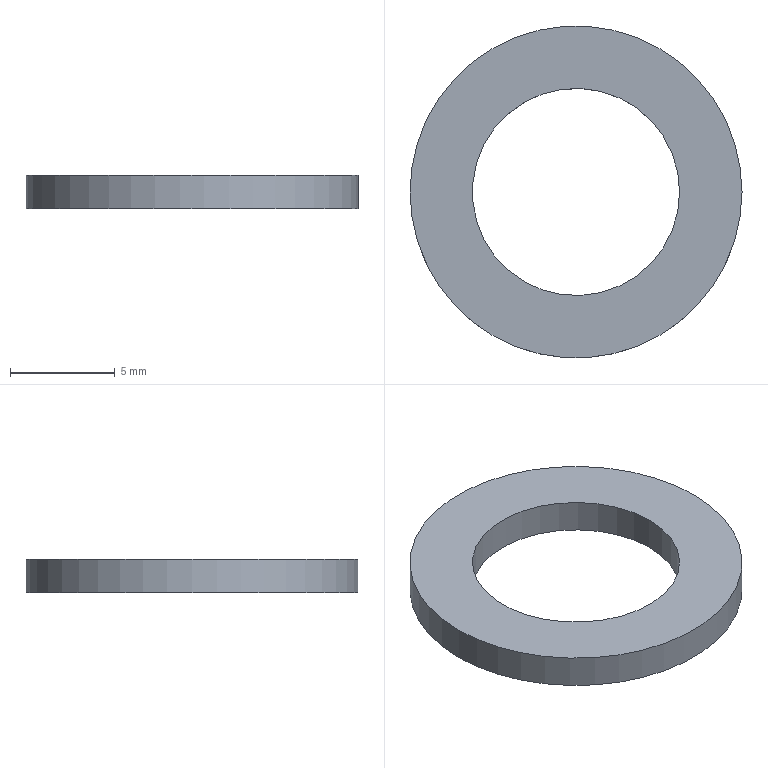Part | NX | features solid 2 | 1 solid | 4 faces | box 15.875 x 15.875 x 1.6 mm | volume 193.404 mm3 | cylinder 2 | plane 2 | commonest cylinder face diameters 9.906 x1 15.875 x1
STEP:
#1=CARTESIAN_POINT('',(7.938,0.,1.6));
#2=VERTEX_POINT('',#1);
#3=CARTESIAN_POINT('',(0.,0.,1.6));
#4=DIRECTION('',(0.,0.,-1.));
#5=DIRECTION('',(1.,0.,0.));
#6=AXIS2_PLACEMENT_3D('',#3,#4,#5);
#7=CIRCLE('',#6,7.938);
#8=EDGE_CURVE('',#2,#2,#7,.T.);
#9=ORIENTED_EDGE('',*,*,#8,.T.);
#10=EDGE_LOOP('',(#9));
#11=FACE_BOUND('',#10,.T.);
#12=CARTESIAN_POINT('',(7.938,0.,0.));
#13=VERTEX_POINT('',#12);
#14=CARTESIAN_POINT('',(0.,0.,0.));
#15=DIRECTION('',(0.,0.,-1.));
#16=DIRECTION('',(1.,0.,0.));
#17=AXIS2_PLACEMENT_3D('',#14,#15,#16);
#18=CIRCLE('',#17,7.938);
#19=EDGE_CURVE('',#13,#13,#18,.T.);
#20=ORIENTED_EDGE('',*,*,#19,.F.);
#21=EDGE_LOOP('',(#20));
#22=FACE_BOUND('',#21,.T.);
#23=CARTESIAN_POINT('',(0.,0.,1.6));
#24=DIRECTION('',(0.,0.,-1.));
#25=DIRECTION('',(-1.,0.,0.));
#26=AXIS2_PLACEMENT_3D('',#23,#24,#25);
#27=CYLINDRICAL_SURFACE('',#26,7.938);
#28=ADVANCED_FACE('',(#11,#22),#27,.T.);
#29=CARTESIAN_POINT('',(4.953,0.,1.6));
#30=VERTEX_POINT('',#29);
#31=CARTESIAN_POINT('',(0.,0.,1.6));
#32=DIRECTION('',(0.,0.,-1.));
#33=DIRECTION('',(1.,0.,0.));
#34=AXIS2_PLACEMENT_3D('',#31,#32,#33);
#35=CIRCLE('',#34,4.953);
#36=EDGE_CURVE('',#30,#30,#35,.T.);
#37=ORIENTED_EDGE('',*,*,#36,.F.);
#38=EDGE_LOOP('',(#37));
#39=FACE_BOUND('',#38,.T.);
#40=CARTESIAN_POINT('',(4.953,0.,0.));
#41=VERTEX_POINT('',#40);
#42=CARTESIAN_POINT('',(0.,0.,0.));
#43=DIRECTION('',(0.,0.,-1.));
#44=DIRECTION('',(1.,0.,0.));
#45=AXIS2_PLACEMENT_3D('',#42,#43,#44);
#46=CIRCLE('',#45,4.953);
#47=EDGE_CURVE('',#41,#41,#46,.T.);
#48=ORIENTED_EDGE('',*,*,#47,.T.);
#49=EDGE_LOOP('',(#48));
#50=FACE_BOUND('',#49,.T.);
#51=CARTESIAN_POINT('',(0.,0.,1.6));
#52=DIRECTION('',(0.,0.,-1.));
#53=DIRECTION('',(-1.,0.,0.));
#54=AXIS2_PLACEMENT_3D('',#51,#52,#53);
#55=CYLINDRICAL_SURFACE('',#54,4.953);
#56=ADVANCED_FACE('',(#39,#50),#55,.F.);
#57=ORIENTED_EDGE('',*,*,#8,.F.);
#58=EDGE_LOOP('',(#57));
#59=FACE_BOUND('',#58,.T.);
#60=ORIENTED_EDGE('',*,*,#36,.T.);
#61=EDGE_LOOP('',(#60));
#62=FACE_BOUND('',#61,.T.);
#63=CARTESIAN_POINT('',(0.,0.,1.6));
#64=DIRECTION('',(0.,0.,-1.));
#65=DIRECTION('',(-1.,0.,0.));
#66=AXIS2_PLACEMENT_3D('',#63,#64,#65);
#67=PLANE('',#66);
#68=ADVANCED_FACE('',(#59,#62),#67,.F.);
#69=ORIENTED_EDGE('',*,*,#19,.T.);
#70=EDGE_LOOP('',(#69));
#71=FACE_BOUND('',#70,.T.);
#72=ORIENTED_EDGE('',*,*,#47,.F.);
#73=EDGE_LOOP('',(#72));
#74=FACE_BOUND('',#73,.T.);
#75=CARTESIAN_POINT('',(0.,0.,0.));
#76=DIRECTION('',(0.,0.,-1.));
#77=DIRECTION('',(-1.,0.,0.));
#78=AXIS2_PLACEMENT_3D('',#75,#76,#77);
#79=PLANE('',#78);
#80=ADVANCED_FACE('',(#71,#74),#79,.T.);
#81=CLOSED_SHELL('',(#28,#56,#68,#80));
#82=MANIFOLD_SOLID_BREP('',#81);
#83=(LENGTH_UNIT()NAMED_UNIT(*)SI_UNIT(.MILLI.,.METRE.));
#84=UNCERTAINTY_MEASURE_WITH_UNIT(LENGTH_MEASURE(0.00001),#83,'','');
#85=(NAMED_UNIT(*)PLANE_ANGLE_UNIT()SI_UNIT($,.RADIAN.));
#86=(NAMED_UNIT(*)SI_UNIT($,.STERADIAN.)SOLID_ANGLE_UNIT());
#87=(GEOMETRIC_REPRESENTATION_CONTEXT(3)GLOBAL_UNCERTAINTY_ASSIGNED_CONTEXT((#84))GLOBAL_UNIT_ASSIGNED_CONTEXT((#83,#85,#86))REPRESENTATION_CONTEXT('',''));
#88=ADVANCED_BREP_SHAPE_REPRESENTATION('',(#82),#87);